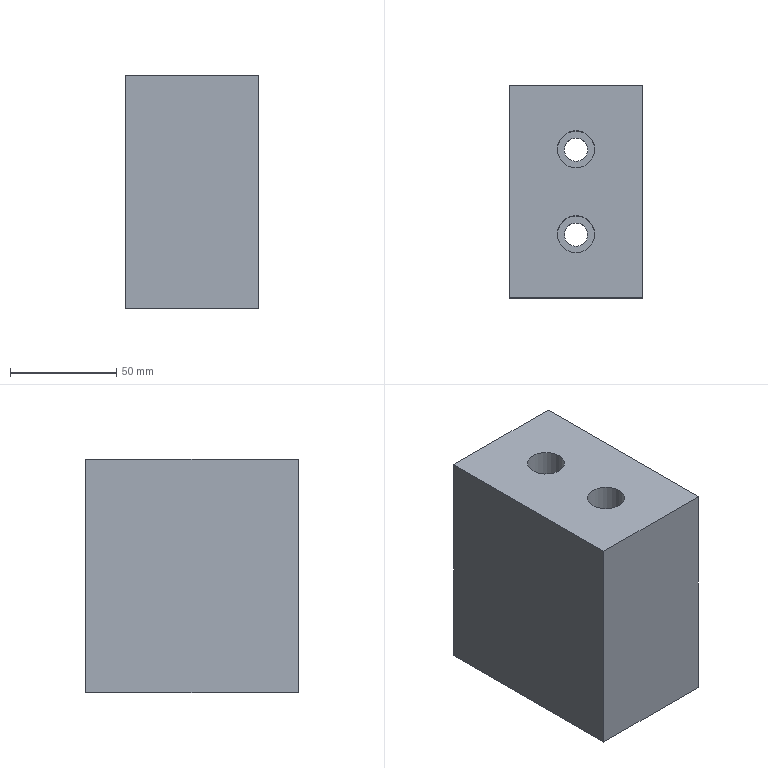Part | NX | features solid 2 | 1 solid | 12 faces | box 63 x 100 x 110 mm | volume 645904 mm3 | plane 8 | cylinder 4 | commonest cylinder face diameters 11 x2 17.5 x2
STEP:
#1=CARTESIAN_POINT('',(1386.25,531.5,120.));
#2=VERTEX_POINT('',#1);
#3=CARTESIAN_POINT('',(1395.,531.5,120.));
#4=DIRECTION('',(0.,0.,1.));
#5=DIRECTION('',(-1.,0.,0.));
#6=AXIS2_PLACEMENT_3D('',#3,#4,#5);
#7=CIRCLE('',#6,8.75);
#8=EDGE_CURVE('',#2,#2,#7,.T.);
#9=ORIENTED_EDGE('',*,*,#8,.F.);
#10=EDGE_LOOP('',(#9));
#11=FACE_BOUND('',#10,.T.);
#12=CARTESIAN_POINT('',(1386.25,491.5,120.));
#13=VERTEX_POINT('',#12);
#14=CARTESIAN_POINT('',(1395.,491.5,120.));
#15=DIRECTION('',(0.,0.,1.));
#16=DIRECTION('',(-1.,0.,0.));
#17=AXIS2_PLACEMENT_3D('',#14,#15,#16);
#18=CIRCLE('',#17,8.75);
#19=EDGE_CURVE('',#13,#13,#18,.T.);
#20=ORIENTED_EDGE('',*,*,#19,.F.);
#21=EDGE_LOOP('',(#20));
#22=FACE_BOUND('',#21,.T.);
#23=CARTESIAN_POINT('',(1426.5,561.5,120.));
#24=VERTEX_POINT('',#23);
#25=CARTESIAN_POINT('',(1363.5,561.5,120.));
#26=VERTEX_POINT('',#25);
#27=CARTESIAN_POINT('',(1443.5,561.5,120.));
#28=DIRECTION('',(-1.,0.,0.));
#29=VECTOR('',#28,1000.);
#30=LINE('',#27,#29);
#31=EDGE_CURVE('',#24,#26,#30,.T.);
#32=ORIENTED_EDGE('',*,*,#31,.T.);
#33=CARTESIAN_POINT('',(1363.5,461.5,120.));
#34=VERTEX_POINT('',#33);
#35=CARTESIAN_POINT('',(1363.5,451.5,120.));
#36=DIRECTION('',(0.,1.,0.));
#37=VECTOR('',#36,1000.);
#38=LINE('',#35,#37);
#39=EDGE_CURVE('',#34,#26,#38,.T.);
#40=ORIENTED_EDGE('',*,*,#39,.F.);
#41=CARTESIAN_POINT('',(1426.5,461.5,120.));
#42=VERTEX_POINT('',#41);
#43=CARTESIAN_POINT('',(1443.5,461.5,120.));
#44=DIRECTION('',(1.,0.,0.));
#45=VECTOR('',#44,1000.);
#46=LINE('',#43,#45);
#47=EDGE_CURVE('',#42,#34,#46,.F.);
#48=ORIENTED_EDGE('',*,*,#47,.F.);
#49=CARTESIAN_POINT('',(1426.5,451.5,120.));
#50=DIRECTION('',(0.,1.,0.));
#51=VECTOR('',#50,1000.);
#52=LINE('',#49,#51);
#53=EDGE_CURVE('',#42,#24,#52,.T.);
#54=ORIENTED_EDGE('',*,*,#53,.T.);
#55=EDGE_LOOP('',(#32,#40,#48,#54));
#56=FACE_BOUND('',#55,.T.);
#57=CARTESIAN_POINT('',(1443.5,451.5,120.));
#58=DIRECTION('',(0.,0.,1.));
#59=DIRECTION('',(0.,1.,0.));
#60=AXIS2_PLACEMENT_3D('',#57,#58,#59);
#61=PLANE('',#60);
#62=ADVANCED_FACE('',(#11,#22,#56),#61,.T.);
#63=ORIENTED_EDGE('',*,*,#47,.T.);
#64=CARTESIAN_POINT('',(1363.5,461.5,10.));
#65=VERTEX_POINT('',#64);
#66=CARTESIAN_POINT('',(1363.5,461.5,120.));
#67=DIRECTION('',(0.,0.,1.));
#68=VECTOR('',#67,1000.);
#69=LINE('',#66,#68);
#70=EDGE_CURVE('',#34,#65,#69,.F.);
#71=ORIENTED_EDGE('',*,*,#70,.T.);
#72=CARTESIAN_POINT('',(1426.5,461.5,10.));
#73=VERTEX_POINT('',#72);
#74=CARTESIAN_POINT('',(1443.5,461.5,10.));
#75=DIRECTION('',(-1.,0.,0.));
#76=VECTOR('',#75,1000.);
#77=LINE('',#74,#76);
#78=EDGE_CURVE('',#73,#65,#77,.T.);
#79=ORIENTED_EDGE('',*,*,#78,.F.);
#80=CARTESIAN_POINT('',(1426.5,461.5,120.));
#81=DIRECTION('',(0.,0.,1.));
#82=VECTOR('',#81,1000.);
#83=LINE('',#80,#82);
#84=EDGE_CURVE('',#42,#73,#83,.F.);
#85=ORIENTED_EDGE('',*,*,#84,.F.);
#86=EDGE_LOOP('',(#63,#71,#79,#85));
#87=FACE_BOUND('',#86,.T.);
#88=CARTESIAN_POINT('',(1443.5,461.5,120.));
#89=DIRECTION('',(0.,1.,0.));
#90=DIRECTION('',(0.,0.,-1.));
#91=AXIS2_PLACEMENT_3D('',#88,#89,#90);
#92=PLANE('',#91);
#93=ADVANCED_FACE('',(#87),#92,.F.);
#94=CARTESIAN_POINT('',(1400.5,531.5,10.));
#95=VERTEX_POINT('',#94);
#96=CARTESIAN_POINT('',(1395.,531.5,10.));
#97=DIRECTION('',(0.,0.,-1.));
#98=DIRECTION('',(1.,0.,0.));
#99=AXIS2_PLACEMENT_3D('',#96,#97,#98);
#100=CIRCLE('',#99,5.5);
#101=EDGE_CURVE('',#95,#95,#100,.F.);
#102=ORIENTED_EDGE('',*,*,#101,.T.);
#103=EDGE_LOOP('',(#102));
#104=FACE_BOUND('',#103,.T.);
#105=CARTESIAN_POINT('',(1400.5,491.5,10.));
#106=VERTEX_POINT('',#105);
#107=CARTESIAN_POINT('',(1395.,491.5,10.));
#108=DIRECTION('',(0.,0.,-1.));
#109=DIRECTION('',(1.,0.,0.));
#110=AXIS2_PLACEMENT_3D('',#107,#108,#109);
#111=CIRCLE('',#110,5.5);
#112=EDGE_CURVE('',#106,#106,#111,.F.);
#113=ORIENTED_EDGE('',*,*,#112,.T.);
#114=EDGE_LOOP('',(#113));
#115=FACE_BOUND('',#114,.T.);
#116=ORIENTED_EDGE('',*,*,#78,.T.);
#117=CARTESIAN_POINT('',(1363.5,561.5,10.));
#118=VERTEX_POINT('',#117);
#119=CARTESIAN_POINT('',(1363.5,451.5,10.));
#120=DIRECTION('',(0.,-1.,0.));
#121=VECTOR('',#120,1000.);
#122=LINE('',#119,#121);
#123=EDGE_CURVE('',#65,#118,#122,.F.);
#124=ORIENTED_EDGE('',*,*,#123,.T.);
#125=CARTESIAN_POINT('',(1426.5,561.5,10.));
#126=VERTEX_POINT('',#125);
#127=CARTESIAN_POINT('',(1443.5,561.5,10.));
#128=DIRECTION('',(1.,0.,0.));
#129=VECTOR('',#128,1000.);
#130=LINE('',#127,#129);
#131=EDGE_CURVE('',#126,#118,#130,.F.);
#132=ORIENTED_EDGE('',*,*,#131,.F.);
#133=CARTESIAN_POINT('',(1426.5,451.5,10.));
#134=DIRECTION('',(0.,-1.,0.));
#135=VECTOR('',#134,1000.);
#136=LINE('',#133,#135);
#137=EDGE_CURVE('',#73,#126,#136,.F.);
#138=ORIENTED_EDGE('',*,*,#137,.F.);
#139=EDGE_LOOP('',(#116,#124,#132,#138));
#140=FACE_BOUND('',#139,.T.);
#141=CARTESIAN_POINT('',(1443.5,451.5,10.));
#142=DIRECTION('',(0.,0.,1.));
#143=DIRECTION('',(0.,1.,0.));
#144=AXIS2_PLACEMENT_3D('',#141,#142,#143);
#145=PLANE('',#144);
#146=ADVANCED_FACE('',(#104,#115,#140),#145,.F.);
#147=CARTESIAN_POINT('',(1426.5,561.5,120.));
#148=DIRECTION('',(0.,0.,-1.));
#149=VECTOR('',#148,1000.);
#150=LINE('',#147,#149);
#151=EDGE_CURVE('',#24,#126,#150,.T.);
#152=ORIENTED_EDGE('',*,*,#151,.T.);
#153=ORIENTED_EDGE('',*,*,#131,.T.);
#154=CARTESIAN_POINT('',(1363.5,561.5,120.));
#155=DIRECTION('',(0.,0.,-1.));
#156=VECTOR('',#155,1000.);
#157=LINE('',#154,#156);
#158=EDGE_CURVE('',#26,#118,#157,.T.);
#159=ORIENTED_EDGE('',*,*,#158,.F.);
#160=ORIENTED_EDGE('',*,*,#31,.F.);
#161=EDGE_LOOP('',(#152,#153,#159,#160));
#162=FACE_BOUND('',#161,.T.);
#163=CARTESIAN_POINT('',(1443.5,561.5,120.));
#164=DIRECTION('',(0.,1.,0.));
#165=DIRECTION('',(0.,0.,-1.));
#166=AXIS2_PLACEMENT_3D('',#163,#164,#165);
#167=PLANE('',#166);
#168=ADVANCED_FACE('',(#162),#167,.T.);
#169=ORIENTED_EDGE('',*,*,#123,.F.);
#170=ORIENTED_EDGE('',*,*,#70,.F.);
#171=ORIENTED_EDGE('',*,*,#39,.T.);
#172=ORIENTED_EDGE('',*,*,#158,.T.);
#173=EDGE_LOOP('',(#169,#170,#171,#172));
#174=FACE_BOUND('',#173,.T.);
#175=CARTESIAN_POINT('',(1363.5,451.5,120.));
#176=DIRECTION('',(1.,0.,0.));
#177=DIRECTION('',(0.,0.,-1.));
#178=AXIS2_PLACEMENT_3D('',#175,#176,#177);
#179=PLANE('',#178);
#180=ADVANCED_FACE('',(#174),#179,.F.);
#181=ORIENTED_EDGE('',*,*,#137,.T.);
#182=ORIENTED_EDGE('',*,*,#151,.F.);
#183=ORIENTED_EDGE('',*,*,#53,.F.);
#184=ORIENTED_EDGE('',*,*,#84,.T.);
#185=EDGE_LOOP('',(#181,#182,#183,#184));
#186=FACE_BOUND('',#185,.T.);
#187=CARTESIAN_POINT('',(1426.5,451.5,120.));
#188=DIRECTION('',(1.,0.,0.));
#189=DIRECTION('',(0.,0.,-1.));
#190=AXIS2_PLACEMENT_3D('',#187,#188,#189);
#191=PLANE('',#190);
#192=ADVANCED_FACE('',(#186),#191,.T.);
#193=ORIENTED_EDGE('',*,*,#112,.F.);
#194=EDGE_LOOP('',(#193));
#195=FACE_BOUND('',#194,.T.);
#196=CARTESIAN_POINT('',(1389.5,491.5,30.));
#197=VERTEX_POINT('',#196);
#198=CARTESIAN_POINT('',(1395.,491.5,30.));
#199=DIRECTION('',(0.,0.,1.));
#200=DIRECTION('',(-1.,0.,0.));
#201=AXIS2_PLACEMENT_3D('',#198,#199,#200);
#202=CIRCLE('',#201,5.5);
#203=EDGE_CURVE('',#197,#197,#202,.T.);
#204=ORIENTED_EDGE('',*,*,#203,.T.);
#205=EDGE_LOOP('',(#204));
#206=FACE_BOUND('',#205,.T.);
#207=CARTESIAN_POINT('',(1395.,491.5,-180.));
#208=DIRECTION('',(0.,0.,-1.));
#209=DIRECTION('',(-1.,0.,0.));
#210=AXIS2_PLACEMENT_3D('',#207,#208,#209);
#211=CYLINDRICAL_SURFACE('',#210,5.5);
#212=ADVANCED_FACE('',(#195,#206),#211,.F.);
#213=ORIENTED_EDGE('',*,*,#203,.F.);
#214=EDGE_LOOP('',(#213));
#215=FACE_BOUND('',#214,.T.);
#216=CARTESIAN_POINT('',(1386.25,491.5,30.));
#217=VERTEX_POINT('',#216);
#218=CARTESIAN_POINT('',(1395.,491.5,30.));
#219=DIRECTION('',(0.,0.,1.));
#220=DIRECTION('',(-1.,0.,0.));
#221=AXIS2_PLACEMENT_3D('',#218,#219,#220);
#222=CIRCLE('',#221,8.75);
#223=EDGE_CURVE('',#217,#217,#222,.T.);
#224=ORIENTED_EDGE('',*,*,#223,.T.);
#225=EDGE_LOOP('',(#224));
#226=FACE_BOUND('',#225,.T.);
#227=CARTESIAN_POINT('',(1403.5,491.5,30.));
#228=DIRECTION('',(0.,0.,-1.));
#229=DIRECTION('',(-1.,0.,0.));
#230=AXIS2_PLACEMENT_3D('',#227,#228,#229);
#231=PLANE('',#230);
#232=ADVANCED_FACE('',(#215,#226),#231,.F.);
#233=ORIENTED_EDGE('',*,*,#223,.F.);
#234=EDGE_LOOP('',(#233));
#235=FACE_BOUND('',#234,.T.);
#236=ORIENTED_EDGE('',*,*,#19,.T.);
#237=EDGE_LOOP('',(#236));
#238=FACE_BOUND('',#237,.T.);
#239=CARTESIAN_POINT('',(1395.,491.5,120.));
#240=DIRECTION('',(0.,0.,-1.));
#241=DIRECTION('',(-1.,0.,0.));
#242=AXIS2_PLACEMENT_3D('',#239,#240,#241);
#243=CYLINDRICAL_SURFACE('',#242,8.75);
#244=ADVANCED_FACE('',(#235,#238),#243,.F.);
#245=ORIENTED_EDGE('',*,*,#101,.F.);
#246=EDGE_LOOP('',(#245));
#247=FACE_BOUND('',#246,.T.);
#248=CARTESIAN_POINT('',(1389.5,531.5,30.));
#249=VERTEX_POINT('',#248);
#250=CARTESIAN_POINT('',(1395.,531.5,30.));
#251=DIRECTION('',(0.,0.,1.));
#252=DIRECTION('',(-1.,0.,0.));
#253=AXIS2_PLACEMENT_3D('',#250,#251,#252);
#254=CIRCLE('',#253,5.5);
#255=EDGE_CURVE('',#249,#249,#254,.T.);
#256=ORIENTED_EDGE('',*,*,#255,.T.);
#257=EDGE_LOOP('',(#256));
#258=FACE_BOUND('',#257,.T.);
#259=CARTESIAN_POINT('',(1395.,531.5,-180.));
#260=DIRECTION('',(0.,0.,-1.));
#261=DIRECTION('',(-1.,0.,0.));
#262=AXIS2_PLACEMENT_3D('',#259,#260,#261);
#263=CYLINDRICAL_SURFACE('',#262,5.5);
#264=ADVANCED_FACE('',(#247,#258),#263,.F.);
#265=ORIENTED_EDGE('',*,*,#255,.F.);
#266=EDGE_LOOP('',(#265));
#267=FACE_BOUND('',#266,.T.);
#268=CARTESIAN_POINT('',(1386.25,531.5,30.));
#269=VERTEX_POINT('',#268);
#270=CARTESIAN_POINT('',(1395.,531.5,30.));
#271=DIRECTION('',(0.,0.,1.));
#272=DIRECTION('',(-1.,0.,0.));
#273=AXIS2_PLACEMENT_3D('',#270,#271,#272);
#274=CIRCLE('',#273,8.75);
#275=EDGE_CURVE('',#269,#269,#274,.T.);
#276=ORIENTED_EDGE('',*,*,#275,.T.);
#277=EDGE_LOOP('',(#276));
#278=FACE_BOUND('',#277,.T.);
#279=CARTESIAN_POINT('',(1403.5,531.5,30.));
#280=DIRECTION('',(0.,0.,-1.));
#281=DIRECTION('',(-1.,0.,0.));
#282=AXIS2_PLACEMENT_3D('',#279,#280,#281);
#283=PLANE('',#282);
#284=ADVANCED_FACE('',(#267,#278),#283,.F.);
#285=ORIENTED_EDGE('',*,*,#275,.F.);
#286=EDGE_LOOP('',(#285));
#287=FACE_BOUND('',#286,.T.);
#288=ORIENTED_EDGE('',*,*,#8,.T.);
#289=EDGE_LOOP('',(#288));
#290=FACE_BOUND('',#289,.T.);
#291=CARTESIAN_POINT('',(1395.,531.5,120.));
#292=DIRECTION('',(0.,0.,-1.));
#293=DIRECTION('',(-1.,0.,0.));
#294=AXIS2_PLACEMENT_3D('',#291,#292,#293);
#295=CYLINDRICAL_SURFACE('',#294,8.75);
#296=ADVANCED_FACE('',(#287,#290),#295,.F.);
#297=CLOSED_SHELL('',(#62,#93,#146,#168,#180,#192,#212,#232,#244,#264,#284,#296));
#298=MANIFOLD_SOLID_BREP('',#297);
#299=(LENGTH_UNIT()NAMED_UNIT(*)SI_UNIT(.MILLI.,.METRE.));
#300=UNCERTAINTY_MEASURE_WITH_UNIT(LENGTH_MEASURE(0.00001),#299,'','');
#301=(NAMED_UNIT(*)PLANE_ANGLE_UNIT()SI_UNIT($,.RADIAN.));
#302=(NAMED_UNIT(*)SI_UNIT($,.STERADIAN.)SOLID_ANGLE_UNIT());
#303=(GEOMETRIC_REPRESENTATION_CONTEXT(3)GLOBAL_UNCERTAINTY_ASSIGNED_CONTEXT((#300))GLOBAL_UNIT_ASSIGNED_CONTEXT((#299,#301,#302))REPRESENTATION_CONTEXT('',''));
#304=ADVANCED_BREP_SHAPE_REPRESENTATION('',(#298),#303);